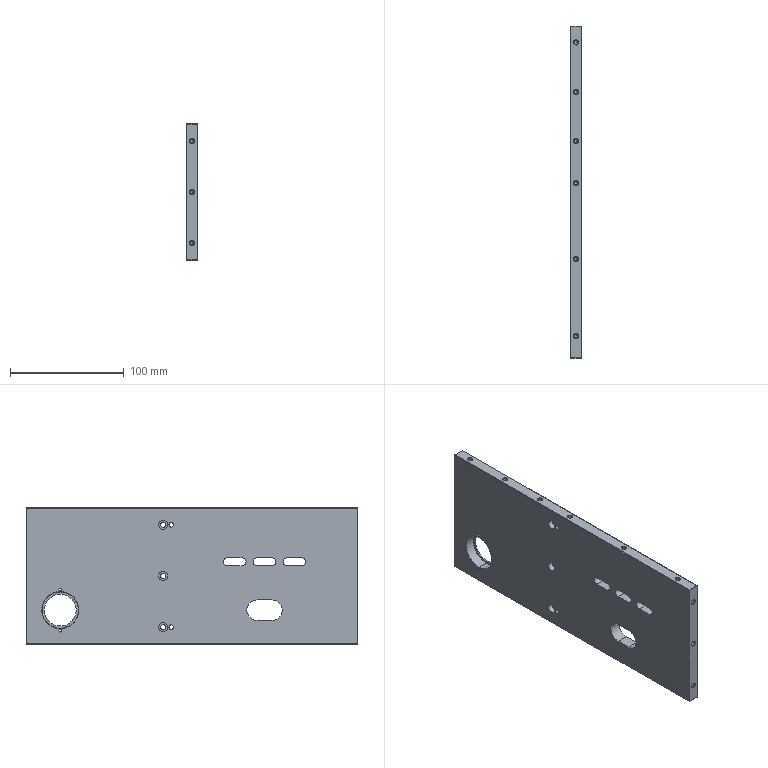Part | NX | 1 solid | 204 faces | box 10 x 291.5 x 120 mm | volume 330143 mm3 | cylinder 100 | cone 74 | plane 30 | commonest cylinder face diameters 3.3 x64 7 x9 4.5 x6 8 x6 2.5 x4 4 x4